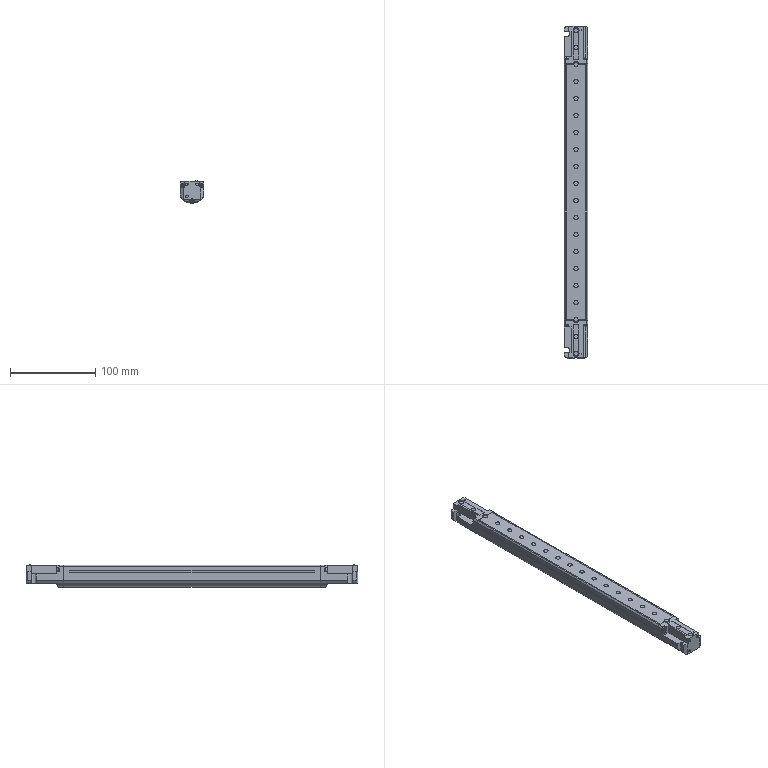Part | STEP file | Guide wheel mechanism revised.sldasm-Part-35 | 1 solid | 302 faces | box 28 x 390 x 26.2 mm | volume 238924 mm3 | cylinder 151 | plane 139 | spline 12 | commonest cylinder face diameters 5 x44 0.5 x12 3 x12 4.5 x12 4.9 x12 32 x11